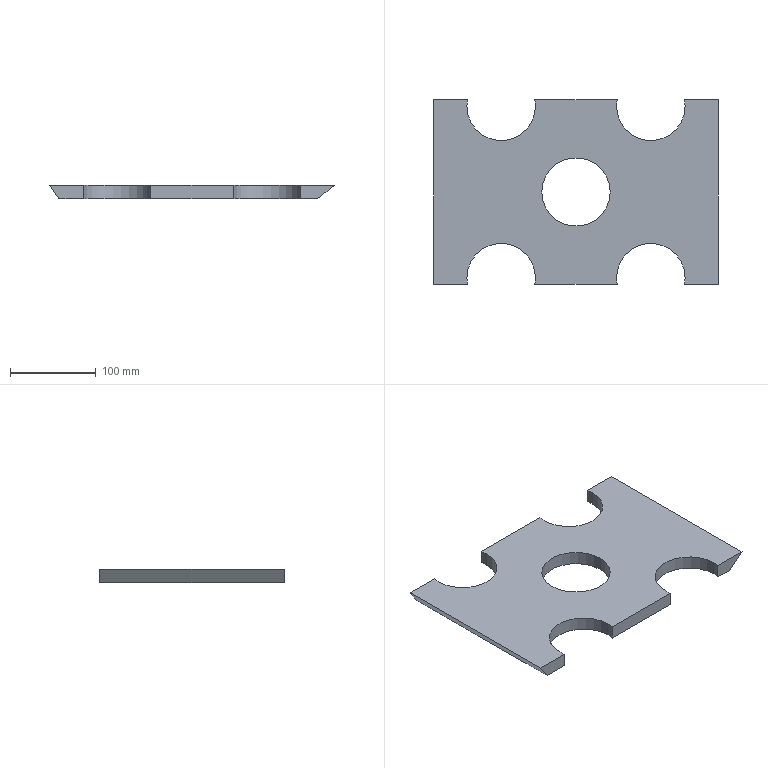Part | SolidWorks | features Extrusion 1, ICE 1 | 1 solid | 24 faces | box 333 x 216 x 16 mm | volume 816357 mm3 | cylinder 14 | plane 10 | commonest cylinder face diameters 80 x14
STEP:
#1=CARTESIAN_POINT('',(126.5,108.,16.));
#2=VERTEX_POINT('',#1);
#3=CARTESIAN_POINT('',(206.5,108.,16.));
#4=VERTEX_POINT('',#3);
#5=CARTESIAN_POINT('',(166.5,108.,16.));
#6=DIRECTION('',(0.,0.,1.));
#7=DIRECTION('',(1.,0.,0.));
#8=AXIS2_PLACEMENT_3D('',#5,#6,#7);
#9=CIRCLE('',#8,40.);
#10=EDGE_CURVE('',#2,#4,#9,.T.);
#11=ORIENTED_EDGE('',*,*,#10,.T.);
#12=CARTESIAN_POINT('',(206.5,108.,0.));
#13=VERTEX_POINT('',#12);
#14=CARTESIAN_POINT('',(206.5,108.,16.));
#15=DIRECTION('',(0.,0.,-1.));
#16=VECTOR('',#15,1000.);
#17=LINE('',#14,#16);
#18=EDGE_CURVE('',#4,#13,#17,.T.);
#19=ORIENTED_EDGE('',*,*,#18,.T.);
#20=CARTESIAN_POINT('',(126.5,108.,0.));
#21=VERTEX_POINT('',#20);
#22=CARTESIAN_POINT('',(166.5,108.,0.));
#23=DIRECTION('',(0.,0.,1.));
#24=DIRECTION('',(1.,0.,0.));
#25=AXIS2_PLACEMENT_3D('',#22,#23,#24);
#26=CIRCLE('',#25,40.);
#27=EDGE_CURVE('',#21,#13,#26,.T.);
#28=ORIENTED_EDGE('',*,*,#27,.F.);
#29=CARTESIAN_POINT('',(126.5,108.,16.));
#30=DIRECTION('',(0.,0.,-1.));
#31=VECTOR('',#30,1000.);
#32=LINE('',#29,#31);
#33=EDGE_CURVE('',#2,#21,#32,.T.);
#34=ORIENTED_EDGE('',*,*,#33,.F.);
#35=EDGE_LOOP('',(#11,#19,#28,#34));
#36=FACE_OUTER_BOUND('',#35,.T.);
#37=CARTESIAN_POINT('',(166.5,108.,16.));
#38=DIRECTION('',(0.,0.,-1.));
#39=DIRECTION('',(-1.,0.,0.));
#40=AXIS2_PLACEMENT_3D('',#37,#38,#39);
#41=CYLINDRICAL_SURFACE('',#40,40.);
#42=ADVANCED_FACE('',(#36),#41,.F.);
#43=CARTESIAN_POINT('',(119.,208.,16.));
#44=VERTEX_POINT('',#43);
#45=CARTESIAN_POINT('',(39.,208.,16.));
#46=VERTEX_POINT('',#45);
#47=CARTESIAN_POINT('',(79.,208.,16.));
#48=DIRECTION('',(0.,0.,-1.));
#49=DIRECTION('',(1.,0.,0.));
#50=AXIS2_PLACEMENT_3D('',#47,#48,#49);
#51=CIRCLE('',#50,40.);
#52=EDGE_CURVE('',#44,#46,#51,.T.);
#53=ORIENTED_EDGE('',*,*,#52,.F.);
#54=CARTESIAN_POINT('',(119.,208.,0.));
#55=VERTEX_POINT('',#54);
#56=CARTESIAN_POINT('',(119.,208.,16.));
#57=DIRECTION('',(0.,0.,-1.));
#58=VECTOR('',#57,1000.);
#59=LINE('',#56,#58);
#60=EDGE_CURVE('',#44,#55,#59,.T.);
#61=ORIENTED_EDGE('',*,*,#60,.T.);
#62=CARTESIAN_POINT('',(39.,208.,0.));
#63=VERTEX_POINT('',#62);
#64=CARTESIAN_POINT('',(79.,208.,0.));
#65=DIRECTION('',(0.,0.,-1.));
#66=DIRECTION('',(1.,0.,0.));
#67=AXIS2_PLACEMENT_3D('',#64,#65,#66);
#68=CIRCLE('',#67,40.);
#69=EDGE_CURVE('',#55,#63,#68,.T.);
#70=ORIENTED_EDGE('',*,*,#69,.T.);
#71=CARTESIAN_POINT('',(39.,208.,16.));
#72=DIRECTION('',(0.,0.,-1.));
#73=VECTOR('',#72,1000.);
#74=LINE('',#71,#73);
#75=EDGE_CURVE('',#46,#63,#74,.T.);
#76=ORIENTED_EDGE('',*,*,#75,.F.);
#77=EDGE_LOOP('',(#53,#61,#70,#76));
#78=FACE_OUTER_BOUND('',#77,.T.);
#79=CARTESIAN_POINT('',(79.,208.,16.));
#80=DIRECTION('',(0.,0.,-1.));
#81=DIRECTION('',(-1.,0.,0.));
#82=AXIS2_PLACEMENT_3D('',#79,#80,#81);
#83=CYLINDRICAL_SURFACE('',#82,40.);
#84=ADVANCED_FACE('',(#78),#83,.F.);
#85=CARTESIAN_POINT('',(39.808,216.,16.));
#86=VERTEX_POINT('',#85);
#87=CARTESIAN_POINT('',(79.,208.,16.));
#88=DIRECTION('',(0.,0.,-1.));
#89=DIRECTION('',(1.,0.,0.));
#90=AXIS2_PLACEMENT_3D('',#87,#88,#89);
#91=CIRCLE('',#90,40.);
#92=EDGE_CURVE('',#46,#86,#91,.T.);
#93=ORIENTED_EDGE('',*,*,#92,.F.);
#94=ORIENTED_EDGE('',*,*,#75,.T.);
#95=CARTESIAN_POINT('',(39.808,216.,0.));
#96=VERTEX_POINT('',#95);
#97=CARTESIAN_POINT('',(79.,208.,0.));
#98=DIRECTION('',(0.,0.,-1.));
#99=DIRECTION('',(1.,0.,0.));
#100=AXIS2_PLACEMENT_3D('',#97,#98,#99);
#101=CIRCLE('',#100,40.);
#102=EDGE_CURVE('',#63,#96,#101,.T.);
#103=ORIENTED_EDGE('',*,*,#102,.T.);
#104=CARTESIAN_POINT('',(39.808,216.,16.));
#105=DIRECTION('',(0.,0.,-1.));
#106=VECTOR('',#105,1000.);
#107=LINE('',#104,#106);
#108=EDGE_CURVE('',#86,#96,#107,.T.);
#109=ORIENTED_EDGE('',*,*,#108,.F.);
#110=EDGE_LOOP('',(#93,#94,#103,#109));
#111=FACE_OUTER_BOUND('',#110,.T.);
#112=CARTESIAN_POINT('',(79.,208.,16.));
#113=DIRECTION('',(0.,0.,-1.));
#114=DIRECTION('',(-1.,0.,0.));
#115=AXIS2_PLACEMENT_3D('',#112,#113,#114);
#116=CYLINDRICAL_SURFACE('',#115,40.);
#117=ADVANCED_FACE('',(#111),#116,.F.);
#118=CARTESIAN_POINT('',(294.,208.,16.));
#119=VERTEX_POINT('',#118);
#120=CARTESIAN_POINT('',(214.,208.,16.));
#121=VERTEX_POINT('',#120);
#122=CARTESIAN_POINT('',(254.,208.,16.));
#123=DIRECTION('',(0.,0.,-1.));
#124=DIRECTION('',(1.,0.,0.));
#125=AXIS2_PLACEMENT_3D('',#122,#123,#124);
#126=CIRCLE('',#125,40.);
#127=EDGE_CURVE('',#119,#121,#126,.T.);
#128=ORIENTED_EDGE('',*,*,#127,.F.);
#129=CARTESIAN_POINT('',(294.,208.,0.));
#130=VERTEX_POINT('',#129);
#131=CARTESIAN_POINT('',(294.,208.,16.));
#132=DIRECTION('',(0.,0.,-1.));
#133=VECTOR('',#132,1000.);
#134=LINE('',#131,#133);
#135=EDGE_CURVE('',#119,#130,#134,.T.);
#136=ORIENTED_EDGE('',*,*,#135,.T.);
#137=CARTESIAN_POINT('',(214.,208.,0.));
#138=VERTEX_POINT('',#137);
#139=CARTESIAN_POINT('',(254.,208.,0.));
#140=DIRECTION('',(0.,0.,-1.));
#141=DIRECTION('',(1.,0.,0.));
#142=AXIS2_PLACEMENT_3D('',#139,#140,#141);
#143=CIRCLE('',#142,40.);
#144=EDGE_CURVE('',#130,#138,#143,.T.);
#145=ORIENTED_EDGE('',*,*,#144,.T.);
#146=CARTESIAN_POINT('',(214.,208.,16.));
#147=DIRECTION('',(0.,0.,-1.));
#148=VECTOR('',#147,1000.);
#149=LINE('',#146,#148);
#150=EDGE_CURVE('',#121,#138,#149,.T.);
#151=ORIENTED_EDGE('',*,*,#150,.F.);
#152=EDGE_LOOP('',(#128,#136,#145,#151));
#153=FACE_OUTER_BOUND('',#152,.T.);
#154=CARTESIAN_POINT('',(254.,208.,16.));
#155=DIRECTION('',(0.,0.,-1.));
#156=DIRECTION('',(-1.,0.,0.));
#157=AXIS2_PLACEMENT_3D('',#154,#155,#156);
#158=CYLINDRICAL_SURFACE('',#157,40.);
#159=ADVANCED_FACE('',(#153),#158,.F.);
#160=CARTESIAN_POINT('',(214.808,216.,16.));
#161=VERTEX_POINT('',#160);
#162=CARTESIAN_POINT('',(254.,208.,16.));
#163=DIRECTION('',(0.,0.,-1.));
#164=DIRECTION('',(1.,0.,0.));
#165=AXIS2_PLACEMENT_3D('',#162,#163,#164);
#166=CIRCLE('',#165,40.);
#167=EDGE_CURVE('',#121,#161,#166,.T.);
#168=ORIENTED_EDGE('',*,*,#167,.F.);
#169=ORIENTED_EDGE('',*,*,#150,.T.);
#170=CARTESIAN_POINT('',(214.808,216.,0.));
#171=VERTEX_POINT('',#170);
#172=CARTESIAN_POINT('',(254.,208.,0.));
#173=DIRECTION('',(0.,0.,-1.));
#174=DIRECTION('',(1.,0.,0.));
#175=AXIS2_PLACEMENT_3D('',#172,#173,#174);
#176=CIRCLE('',#175,40.);
#177=EDGE_CURVE('',#138,#171,#176,.T.);
#178=ORIENTED_EDGE('',*,*,#177,.T.);
#179=CARTESIAN_POINT('',(214.808,216.,16.));
#180=DIRECTION('',(0.,0.,-1.));
#181=VECTOR('',#180,1000.);
#182=LINE('',#179,#181);
#183=EDGE_CURVE('',#161,#171,#182,.T.);
#184=ORIENTED_EDGE('',*,*,#183,.F.);
#185=EDGE_LOOP('',(#168,#169,#178,#184));
#186=FACE_OUTER_BOUND('',#185,.T.);
#187=CARTESIAN_POINT('',(254.,208.,16.));
#188=DIRECTION('',(0.,0.,-1.));
#189=DIRECTION('',(-1.,0.,0.));
#190=AXIS2_PLACEMENT_3D('',#187,#188,#189);
#191=CYLINDRICAL_SURFACE('',#190,40.);
#192=ADVANCED_FACE('',(#186),#191,.F.);
#193=CARTESIAN_POINT('',(294.,8.,16.));
#194=VERTEX_POINT('',#193);
#195=CARTESIAN_POINT('',(293.192,0.,16.));
#196=VERTEX_POINT('',#195);
#197=CARTESIAN_POINT('',(254.,8.,16.));
#198=DIRECTION('',(0.,0.,-1.));
#199=DIRECTION('',(1.,0.,0.));
#200=AXIS2_PLACEMENT_3D('',#197,#198,#199);
#201=CIRCLE('',#200,40.);
#202=EDGE_CURVE('',#194,#196,#201,.T.);
#203=ORIENTED_EDGE('',*,*,#202,.F.);
#204=CARTESIAN_POINT('',(294.,8.,0.));
#205=VERTEX_POINT('',#204);
#206=CARTESIAN_POINT('',(294.,8.,16.));
#207=DIRECTION('',(0.,0.,-1.));
#208=VECTOR('',#207,1000.);
#209=LINE('',#206,#208);
#210=EDGE_CURVE('',#194,#205,#209,.T.);
#211=ORIENTED_EDGE('',*,*,#210,.T.);
#212=CARTESIAN_POINT('',(293.192,0.,0.));
#213=VERTEX_POINT('',#212);
#214=CARTESIAN_POINT('',(254.,8.,0.));
#215=DIRECTION('',(0.,0.,-1.));
#216=DIRECTION('',(1.,0.,0.));
#217=AXIS2_PLACEMENT_3D('',#214,#215,#216);
#218=CIRCLE('',#217,40.);
#219=EDGE_CURVE('',#205,#213,#218,.T.);
#220=ORIENTED_EDGE('',*,*,#219,.T.);
#221=CARTESIAN_POINT('',(293.192,0.,16.));
#222=DIRECTION('',(0.,0.,-1.));
#223=VECTOR('',#222,1000.);
#224=LINE('',#221,#223);
#225=EDGE_CURVE('',#196,#213,#224,.T.);
#226=ORIENTED_EDGE('',*,*,#225,.F.);
#227=EDGE_LOOP('',(#203,#211,#220,#226));
#228=FACE_OUTER_BOUND('',#227,.T.);
#229=CARTESIAN_POINT('',(254.,8.,16.));
#230=DIRECTION('',(0.,0.,-1.));
#231=DIRECTION('',(-1.,0.,0.));
#232=AXIS2_PLACEMENT_3D('',#229,#230,#231);
#233=CYLINDRICAL_SURFACE('',#232,40.);
#234=ADVANCED_FACE('',(#228),#233,.F.);
#235=ORIENTED_EDGE('',*,*,#210,.F.);
#236=CARTESIAN_POINT('',(214.,8.,16.));
#237=VERTEX_POINT('',#236);
#238=CARTESIAN_POINT('',(254.,8.,16.));
#239=DIRECTION('',(0.,0.,-1.));
#240=DIRECTION('',(1.,0.,0.));
#241=AXIS2_PLACEMENT_3D('',#238,#239,#240);
#242=CIRCLE('',#241,40.);
#243=EDGE_CURVE('',#237,#194,#242,.T.);
#244=ORIENTED_EDGE('',*,*,#243,.F.);
#245=CARTESIAN_POINT('',(214.,8.,0.));
#246=VERTEX_POINT('',#245);
#247=CARTESIAN_POINT('',(214.,8.,16.));
#248=DIRECTION('',(0.,0.,-1.));
#249=VECTOR('',#248,1000.);
#250=LINE('',#247,#249);
#251=EDGE_CURVE('',#237,#246,#250,.T.);
#252=ORIENTED_EDGE('',*,*,#251,.T.);
#253=CARTESIAN_POINT('',(254.,8.,0.));
#254=DIRECTION('',(0.,0.,-1.));
#255=DIRECTION('',(1.,0.,0.));
#256=AXIS2_PLACEMENT_3D('',#253,#254,#255);
#257=CIRCLE('',#256,40.);
#258=EDGE_CURVE('',#246,#205,#257,.T.);
#259=ORIENTED_EDGE('',*,*,#258,.T.);
#260=EDGE_LOOP('',(#235,#244,#252,#259));
#261=FACE_OUTER_BOUND('',#260,.T.);
#262=CARTESIAN_POINT('',(254.,8.,16.));
#263=DIRECTION('',(0.,0.,-1.));
#264=DIRECTION('',(-1.,0.,0.));
#265=AXIS2_PLACEMENT_3D('',#262,#263,#264);
#266=CYLINDRICAL_SURFACE('',#265,40.);
#267=ADVANCED_FACE('',(#261),#266,.F.);
#268=CARTESIAN_POINT('',(119.,8.,16.));
#269=VERTEX_POINT('',#268);
#270=CARTESIAN_POINT('',(118.192,0.,16.));
#271=VERTEX_POINT('',#270);
#272=CARTESIAN_POINT('',(79.,8.,16.));
#273=DIRECTION('',(0.,0.,-1.));
#274=DIRECTION('',(1.,0.,0.));
#275=AXIS2_PLACEMENT_3D('',#272,#273,#274);
#276=CIRCLE('',#275,40.);
#277=EDGE_CURVE('',#269,#271,#276,.T.);
#278=ORIENTED_EDGE('',*,*,#277,.F.);
#279=CARTESIAN_POINT('',(119.,8.,0.));
#280=VERTEX_POINT('',#279);
#281=CARTESIAN_POINT('',(119.,8.,16.));
#282=DIRECTION('',(0.,0.,-1.));
#283=VECTOR('',#282,1000.);
#284=LINE('',#281,#283);
#285=EDGE_CURVE('',#269,#280,#284,.T.);
#286=ORIENTED_EDGE('',*,*,#285,.T.);
#287=CARTESIAN_POINT('',(118.192,0.,0.));
#288=VERTEX_POINT('',#287);
#289=CARTESIAN_POINT('',(79.,8.,0.));
#290=DIRECTION('',(0.,0.,-1.));
#291=DIRECTION('',(1.,0.,0.));
#292=AXIS2_PLACEMENT_3D('',#289,#290,#291);
#293=CIRCLE('',#292,40.);
#294=EDGE_CURVE('',#280,#288,#293,.T.);
#295=ORIENTED_EDGE('',*,*,#294,.T.);
#296=CARTESIAN_POINT('',(118.192,0.,16.));
#297=DIRECTION('',(0.,0.,-1.));
#298=VECTOR('',#297,1000.);
#299=LINE('',#296,#298);
#300=EDGE_CURVE('',#271,#288,#299,.T.);
#301=ORIENTED_EDGE('',*,*,#300,.F.);
#302=EDGE_LOOP('',(#278,#286,#295,#301));
#303=FACE_OUTER_BOUND('',#302,.T.);
#304=CARTESIAN_POINT('',(79.,8.,16.));
#305=DIRECTION('',(0.,0.,-1.));
#306=DIRECTION('',(-1.,0.,0.));
#307=AXIS2_PLACEMENT_3D('',#304,#305,#306);
#308=CYLINDRICAL_SURFACE('',#307,40.);
#309=ADVANCED_FACE('',(#303),#308,.F.);
#310=ORIENTED_EDGE('',*,*,#285,.F.);
#311=CARTESIAN_POINT('',(39.,8.,16.));
#312=VERTEX_POINT('',#311);
#313=CARTESIAN_POINT('',(79.,8.,16.));
#314=DIRECTION('',(0.,0.,-1.));
#315=DIRECTION('',(1.,0.,0.));
#316=AXIS2_PLACEMENT_3D('',#313,#314,#315);
#317=CIRCLE('',#316,40.);
#318=EDGE_CURVE('',#312,#269,#317,.T.);
#319=ORIENTED_EDGE('',*,*,#318,.F.);
#320=CARTESIAN_POINT('',(39.,8.,0.));
#321=VERTEX_POINT('',#320);
#322=CARTESIAN_POINT('',(39.,8.,16.));
#323=DIRECTION('',(0.,0.,-1.));
#324=VECTOR('',#323,1000.);
#325=LINE('',#322,#324);
#326=EDGE_CURVE('',#312,#321,#325,.T.);
#327=ORIENTED_EDGE('',*,*,#326,.T.);
#328=CARTESIAN_POINT('',(79.,8.,0.));
#329=DIRECTION('',(0.,0.,-1.));
#330=DIRECTION('',(1.,0.,0.));
#331=AXIS2_PLACEMENT_3D('',#328,#329,#330);
#332=CIRCLE('',#331,40.);
#333=EDGE_CURVE('',#321,#280,#332,.T.);
#334=ORIENTED_EDGE('',*,*,#333,.T.);
#335=EDGE_LOOP('',(#310,#319,#327,#334));
#336=FACE_OUTER_BOUND('',#335,.T.);
#337=CARTESIAN_POINT('',(79.,8.,16.));
#338=DIRECTION('',(0.,0.,-1.));
#339=DIRECTION('',(-1.,0.,0.));
#340=AXIS2_PLACEMENT_3D('',#337,#338,#339);
#341=CYLINDRICAL_SURFACE('',#340,40.);
#342=ADVANCED_FACE('',(#336),#341,.F.);
#343=CARTESIAN_POINT('',(0.,216.,16.));
#344=VERTEX_POINT('',#343);
#345=CARTESIAN_POINT('',(0.,0.,16.));
#346=VERTEX_POINT('',#345);
#347=CARTESIAN_POINT('',(0.,0.,16.));
#348=DIRECTION('',(0.,-1.,0.));
#349=VECTOR('',#348,1000.);
#350=LINE('',#347,#349);
#351=EDGE_CURVE('',#344,#346,#350,.T.);
#352=ORIENTED_EDGE('',*,*,#351,.T.);
#353=CARTESIAN_POINT('',(39.808,0.,16.));
#354=VERTEX_POINT('',#353);
#355=CARTESIAN_POINT('',(0.,0.,16.));
#356=DIRECTION('',(1.,0.,0.));
#357=VECTOR('',#356,1000.);
#358=LINE('',#355,#357);
#359=EDGE_CURVE('',#346,#354,#358,.T.);
#360=ORIENTED_EDGE('',*,*,#359,.T.);
#361=CARTESIAN_POINT('',(79.,8.,16.));
#362=DIRECTION('',(0.,0.,-1.));
#363=DIRECTION('',(1.,0.,0.));
#364=AXIS2_PLACEMENT_3D('',#361,#362,#363);
#365=CIRCLE('',#364,40.);
#366=EDGE_CURVE('',#354,#312,#365,.T.);
#367=ORIENTED_EDGE('',*,*,#366,.T.);
#368=ORIENTED_EDGE('',*,*,#318,.T.);
#369=ORIENTED_EDGE('',*,*,#277,.T.);
#370=CARTESIAN_POINT('',(214.808,0.,16.));
#371=VERTEX_POINT('',#370);
#372=CARTESIAN_POINT('',(118.192,0.,16.));
#373=DIRECTION('',(1.,0.,0.));
#374=VECTOR('',#373,1000.);
#375=LINE('',#372,#374);
#376=EDGE_CURVE('',#271,#371,#375,.T.);
#377=ORIENTED_EDGE('',*,*,#376,.T.);
#378=CARTESIAN_POINT('',(254.,8.,16.));
#379=DIRECTION('',(0.,0.,-1.));
#380=DIRECTION('',(1.,0.,0.));
#381=AXIS2_PLACEMENT_3D('',#378,#379,#380);
#382=CIRCLE('',#381,40.);
#383=EDGE_CURVE('',#371,#237,#382,.T.);
#384=ORIENTED_EDGE('',*,*,#383,.T.);
#385=ORIENTED_EDGE('',*,*,#243,.T.);
#386=ORIENTED_EDGE('',*,*,#202,.T.);
#387=CARTESIAN_POINT('',(333.,0.,16.));
#388=VERTEX_POINT('',#387);
#389=CARTESIAN_POINT('',(293.192,0.,16.));
#390=DIRECTION('',(1.,0.,0.));
#391=VECTOR('',#390,1000.);
#392=LINE('',#389,#391);
#393=EDGE_CURVE('',#196,#388,#392,.T.);
#394=ORIENTED_EDGE('',*,*,#393,.T.);
#395=CARTESIAN_POINT('',(333.,216.,16.));
#396=VERTEX_POINT('',#395);
#397=CARTESIAN_POINT('',(333.,0.,16.));
#398=DIRECTION('',(0.,1.,0.));
#399=VECTOR('',#398,1000.);
#400=LINE('',#397,#399);
#401=EDGE_CURVE('',#388,#396,#400,.T.);
#402=ORIENTED_EDGE('',*,*,#401,.T.);
#403=CARTESIAN_POINT('',(293.192,216.,16.));
#404=VERTEX_POINT('',#403);
#405=CARTESIAN_POINT('',(293.192,216.,16.));
#406=DIRECTION('',(-1.,0.,0.));
#407=VECTOR('',#406,1000.);
#408=LINE('',#405,#407);
#409=EDGE_CURVE('',#396,#404,#408,.T.);
#410=ORIENTED_EDGE('',*,*,#409,.T.);
#411=CARTESIAN_POINT('',(254.,208.,16.));
#412=DIRECTION('',(0.,0.,-1.));
#413=DIRECTION('',(1.,0.,0.));
#414=AXIS2_PLACEMENT_3D('',#411,#412,#413);
#415=CIRCLE('',#414,40.);
#416=EDGE_CURVE('',#404,#119,#415,.T.);
#417=ORIENTED_EDGE('',*,*,#416,.T.);
#418=ORIENTED_EDGE('',*,*,#127,.T.);
#419=ORIENTED_EDGE('',*,*,#167,.T.);
#420=CARTESIAN_POINT('',(118.192,216.,16.));
#421=VERTEX_POINT('',#420);
#422=CARTESIAN_POINT('',(118.192,216.,16.));
#423=DIRECTION('',(-1.,0.,0.));
#424=VECTOR('',#423,1000.);
#425=LINE('',#422,#424);
#426=EDGE_CURVE('',#161,#421,#425,.T.);
#427=ORIENTED_EDGE('',*,*,#426,.T.);
#428=CARTESIAN_POINT('',(79.,208.,16.));
#429=DIRECTION('',(0.,0.,-1.));
#430=DIRECTION('',(1.,0.,0.));
#431=AXIS2_PLACEMENT_3D('',#428,#429,#430);
#432=CIRCLE('',#431,40.);
#433=EDGE_CURVE('',#421,#44,#432,.T.);
#434=ORIENTED_EDGE('',*,*,#433,.T.);
#435=ORIENTED_EDGE('',*,*,#52,.T.);
#436=ORIENTED_EDGE('',*,*,#92,.T.);
#437=CARTESIAN_POINT('',(0.,216.,16.));
#438=DIRECTION('',(-1.,0.,0.));
#439=VECTOR('',#438,1000.);
#440=LINE('',#437,#439);
#441=EDGE_CURVE('',#86,#344,#440,.T.);
#442=ORIENTED_EDGE('',*,*,#441,.T.);
#443=EDGE_LOOP('',(#352,#360,#367,#368,#369,#377,#384,#385,#386,#394,#402,#410,#417,#418,#419,#427,#434,#435,#436,#442));
#444=FACE_OUTER_BOUND('',#443,.T.);
#445=ORIENTED_EDGE('',*,*,#10,.F.);
#446=CARTESIAN_POINT('',(166.5,108.,16.));
#447=DIRECTION('',(0.,0.,1.));
#448=DIRECTION('',(1.,0.,0.));
#449=AXIS2_PLACEMENT_3D('',#446,#447,#448);
#450=CIRCLE('',#449,40.);
#451=EDGE_CURVE('',#4,#2,#450,.T.);
#452=ORIENTED_EDGE('',*,*,#451,.F.);
#453=EDGE_LOOP('',(#445,#452));
#454=FACE_BOUND('',#453,.T.);
#455=CARTESIAN_POINT('',(79.,208.,16.));
#456=DIRECTION('',(0.,0.,1.));
#457=DIRECTION('',(1.,0.,0.));
#458=AXIS2_PLACEMENT_3D('',#455,#456,#457);
#459=PLANE('',#458);
#460=ADVANCED_FACE('',(#444,#454),#459,.T.);
#461=CARTESIAN_POINT('',(313.3,216.,0.));
#462=VERTEX_POINT('',#461);
#463=CARTESIAN_POINT('',(293.192,216.,0.));
#464=VERTEX_POINT('',#463);
#465=CARTESIAN_POINT('',(293.192,216.,0.));
#466=DIRECTION('',(-1.,0.,0.));
#467=VECTOR('',#466,1000.);
#468=LINE('',#465,#467);
#469=EDGE_CURVE('',#462,#464,#468,.T.);
#470=ORIENTED_EDGE('',*,*,#469,.F.);
#471=CARTESIAN_POINT('',(313.3,0.,0.));
#472=VERTEX_POINT('',#471);
#473=CARTESIAN_POINT('',(313.3,216.,0.));
#474=DIRECTION('',(0.,-1.,0.));
#475=VECTOR('',#474,1000.);
#476=LINE('',#473,#475);
#477=EDGE_CURVE('',#462,#472,#476,.T.);
#478=ORIENTED_EDGE('',*,*,#477,.T.);
#479=CARTESIAN_POINT('',(293.192,0.,0.));
#480=DIRECTION('',(1.,0.,0.));
#481=VECTOR('',#480,1000.);
#482=LINE('',#479,#481);
#483=EDGE_CURVE('',#213,#472,#482,.T.);
#484=ORIENTED_EDGE('',*,*,#483,.F.);
#485=ORIENTED_EDGE('',*,*,#219,.F.);
#486=ORIENTED_EDGE('',*,*,#258,.F.);
#487=CARTESIAN_POINT('',(214.808,0.,0.));
#488=VERTEX_POINT('',#487);
#489=CARTESIAN_POINT('',(254.,8.,0.));
#490=DIRECTION('',(0.,0.,-1.));
#491=DIRECTION('',(1.,0.,0.));
#492=AXIS2_PLACEMENT_3D('',#489,#490,#491);
#493=CIRCLE('',#492,40.);
#494=EDGE_CURVE('',#488,#246,#493,.T.);
#495=ORIENTED_EDGE('',*,*,#494,.F.);
#496=CARTESIAN_POINT('',(118.192,0.,0.));
#497=DIRECTION('',(1.,0.,0.));
#498=VECTOR('',#497,1000.);
#499=LINE('',#496,#498);
#500=EDGE_CURVE('',#288,#488,#499,.T.);
#501=ORIENTED_EDGE('',*,*,#500,.F.);
#502=ORIENTED_EDGE('',*,*,#294,.F.);
#503=ORIENTED_EDGE('',*,*,#333,.F.);
#504=CARTESIAN_POINT('',(39.808,0.,0.));
#505=VERTEX_POINT('',#504);
#506=CARTESIAN_POINT('',(79.,8.,0.));
#507=DIRECTION('',(0.,0.,-1.));
#508=DIRECTION('',(1.,0.,0.));
#509=AXIS2_PLACEMENT_3D('',#506,#507,#508);
#510=CIRCLE('',#509,40.);
#511=EDGE_CURVE('',#505,#321,#510,.T.);
#512=ORIENTED_EDGE('',*,*,#511,.F.);
#513=CARTESIAN_POINT('',(10.7,0.,0.));
#514=VERTEX_POINT('',#513);
#515=CARTESIAN_POINT('',(0.,0.,0.));
#516=DIRECTION('',(1.,0.,0.));
#517=VECTOR('',#516,1000.);
#518=LINE('',#515,#517);
#519=EDGE_CURVE('',#514,#505,#518,.T.);
#520=ORIENTED_EDGE('',*,*,#519,.F.);
#521=CARTESIAN_POINT('',(10.7,216.,0.));
#522=VERTEX_POINT('',#521);
#523=CARTESIAN_POINT('',(10.7,216.,0.));
#524=DIRECTION('',(0.,-1.,0.));
#525=VECTOR('',#524,1000.);
#526=LINE('',#523,#525);
#527=EDGE_CURVE('',#522,#514,#526,.T.);
#528=ORIENTED_EDGE('',*,*,#527,.F.);
#529=CARTESIAN_POINT('',(0.,216.,0.));
#530=DIRECTION('',(-1.,0.,0.));
#531=VECTOR('',#530,1000.);
#532=LINE('',#529,#531);
#533=EDGE_CURVE('',#96,#522,#532,.T.);
#534=ORIENTED_EDGE('',*,*,#533,.F.);
#535=ORIENTED_EDGE('',*,*,#102,.F.);
#536=ORIENTED_EDGE('',*,*,#69,.F.);
#537=CARTESIAN_POINT('',(118.192,216.,0.));
#538=VERTEX_POINT('',#537);
#539=CARTESIAN_POINT('',(79.,208.,0.));
#540=DIRECTION('',(0.,0.,-1.));
#541=DIRECTION('',(1.,0.,0.));
#542=AXIS2_PLACEMENT_3D('',#539,#540,#541);
#543=CIRCLE('',#542,40.);
#544=EDGE_CURVE('',#538,#55,#543,.T.);
#545=ORIENTED_EDGE('',*,*,#544,.F.);
#546=CARTESIAN_POINT('',(118.192,216.,0.));
#547=DIRECTION('',(-1.,0.,0.));
#548=VECTOR('',#547,1000.);
#549=LINE('',#546,#548);
#550=EDGE_CURVE('',#171,#538,#549,.T.);
#551=ORIENTED_EDGE('',*,*,#550,.F.);
#552=ORIENTED_EDGE('',*,*,#177,.F.);
#553=ORIENTED_EDGE('',*,*,#144,.F.);
#554=CARTESIAN_POINT('',(254.,208.,0.));
#555=DIRECTION('',(0.,0.,-1.));
#556=DIRECTION('',(1.,0.,0.));
#557=AXIS2_PLACEMENT_3D('',#554,#555,#556);
#558=CIRCLE('',#557,40.);
#559=EDGE_CURVE('',#464,#130,#558,.T.);
#560=ORIENTED_EDGE('',*,*,#559,.F.);
#561=EDGE_LOOP('',(#470,#478,#484,#485,#486,#495,#501,#502,#503,#512,#520,#528,#534,#535,#536,#545,#551,#552,#553,#560));
#562=FACE_OUTER_BOUND('',#561,.T.);
#563=ORIENTED_EDGE('',*,*,#27,.T.);
#564=CARTESIAN_POINT('',(166.5,108.,0.));
#565=DIRECTION('',(0.,0.,1.));
#566=DIRECTION('',(1.,0.,0.));
#567=AXIS2_PLACEMENT_3D('',#564,#565,#566);
#568=CIRCLE('',#567,40.);
#569=EDGE_CURVE('',#13,#21,#568,.T.);
#570=ORIENTED_EDGE('',*,*,#569,.T.);
#571=EDGE_LOOP('',(#563,#570));
#572=FACE_BOUND('',#571,.T.);
#573=CARTESIAN_POINT('',(79.,208.,0.));
#574=DIRECTION('',(0.,0.,1.));
#575=DIRECTION('',(1.,0.,0.));
#576=AXIS2_PLACEMENT_3D('',#573,#574,#575);
#577=PLANE('',#576);
#578=ADVANCED_FACE('',(#562,#572),#577,.F.);
#579=ORIENTED_EDGE('',*,*,#359,.F.);
#580=CARTESIAN_POINT('',(0.,0.,16.));
#581=DIRECTION('',(-0.5559,0.,0.8313));
#582=VECTOR('',#581,1000.);
#583=LINE('',#580,#582);
#584=EDGE_CURVE('',#514,#346,#583,.T.);
#585=ORIENTED_EDGE('',*,*,#584,.F.);
#586=ORIENTED_EDGE('',*,*,#519,.T.);
#587=CARTESIAN_POINT('',(39.808,0.,16.));
#588=DIRECTION('',(0.,0.,-1.));
#589=VECTOR('',#588,1000.);
#590=LINE('',#587,#589);
#591=EDGE_CURVE('',#354,#505,#590,.T.);
#592=ORIENTED_EDGE('',*,*,#591,.F.);
#593=EDGE_LOOP('',(#579,#585,#586,#592));
#594=FACE_OUTER_BOUND('',#593,.T.);
#595=CARTESIAN_POINT('',(0.,0.,16.));
#596=DIRECTION('',(0.,1.,0.));
#597=DIRECTION('',(0.,0.,1.));
#598=AXIS2_PLACEMENT_3D('',#595,#596,#597);
#599=PLANE('',#598);
#600=ADVANCED_FACE('',(#594),#599,.F.);
#601=ORIENTED_EDGE('',*,*,#326,.F.);
#602=ORIENTED_EDGE('',*,*,#366,.F.);
#603=ORIENTED_EDGE('',*,*,#591,.T.);
#604=ORIENTED_EDGE('',*,*,#511,.T.);
#605=EDGE_LOOP('',(#601,#602,#603,#604));
#606=FACE_OUTER_BOUND('',#605,.T.);
#607=CARTESIAN_POINT('',(79.,8.,16.));
#608=DIRECTION('',(0.,0.,-1.));
#609=DIRECTION('',(-1.,0.,0.));
#610=AXIS2_PLACEMENT_3D('',#607,#608,#609);
#611=CYLINDRICAL_SURFACE('',#610,40.);
#612=ADVANCED_FACE('',(#606),#611,.F.);
#613=ORIENTED_EDGE('',*,*,#500,.T.);
#614=CARTESIAN_POINT('',(214.808,0.,16.));
#615=DIRECTION('',(0.,0.,-1.));
#616=VECTOR('',#615,1000.);
#617=LINE('',#614,#616);
#618=EDGE_CURVE('',#371,#488,#617,.T.);
#619=ORIENTED_EDGE('',*,*,#618,.F.);
#620=ORIENTED_EDGE('',*,*,#376,.F.);
#621=ORIENTED_EDGE('',*,*,#300,.T.);
#622=EDGE_LOOP('',(#613,#619,#620,#621));
#623=FACE_OUTER_BOUND('',#622,.T.);
#624=CARTESIAN_POINT('',(118.192,0.,16.));
#625=DIRECTION('',(0.,1.,0.));
#626=DIRECTION('',(0.,0.,1.));
#627=AXIS2_PLACEMENT_3D('',#624,#625,#626);
#628=PLANE('',#627);
#629=ADVANCED_FACE('',(#623),#628,.F.);
#630=ORIENTED_EDGE('',*,*,#251,.F.);
#631=ORIENTED_EDGE('',*,*,#383,.F.);
#632=ORIENTED_EDGE('',*,*,#618,.T.);
#633=ORIENTED_EDGE('',*,*,#494,.T.);
#634=EDGE_LOOP('',(#630,#631,#632,#633));
#635=FACE_OUTER_BOUND('',#634,.T.);
#636=CARTESIAN_POINT('',(254.,8.,16.));
#637=DIRECTION('',(0.,0.,-1.));
#638=DIRECTION('',(-1.,0.,0.));
#639=AXIS2_PLACEMENT_3D('',#636,#637,#638);
#640=CYLINDRICAL_SURFACE('',#639,40.);
#641=ADVANCED_FACE('',(#635),#640,.F.);
#642=ORIENTED_EDGE('',*,*,#483,.T.);
#643=CARTESIAN_POINT('',(333.,0.,16.));
#644=DIRECTION('',(-0.7762,0.,-0.6304));
#645=VECTOR('',#644,1000.);
#646=LINE('',#643,#645);
#647=EDGE_CURVE('',#388,#472,#646,.T.);
#648=ORIENTED_EDGE('',*,*,#647,.F.);
#649=ORIENTED_EDGE('',*,*,#393,.F.);
#650=ORIENTED_EDGE('',*,*,#225,.T.);
#651=EDGE_LOOP('',(#642,#648,#649,#650));
#652=FACE_OUTER_BOUND('',#651,.T.);
#653=CARTESIAN_POINT('',(293.192,0.,16.));
#654=DIRECTION('',(0.,1.,0.));
#655=DIRECTION('',(0.,0.,1.));
#656=AXIS2_PLACEMENT_3D('',#653,#654,#655);
#657=PLANE('',#656);
#658=ADVANCED_FACE('',(#652),#657,.F.);
#659=ORIENTED_EDGE('',*,*,#409,.F.);
#660=CARTESIAN_POINT('',(333.,216.,16.));
#661=DIRECTION('',(-0.7762,0.,-0.6304));
#662=VECTOR('',#661,1000.);
#663=LINE('',#660,#662);
#664=EDGE_CURVE('',#396,#462,#663,.T.);
#665=ORIENTED_EDGE('',*,*,#664,.T.);
#666=ORIENTED_EDGE('',*,*,#469,.T.);
#667=CARTESIAN_POINT('',(293.192,216.,16.));
#668=DIRECTION('',(0.,0.,-1.));
#669=VECTOR('',#668,1000.);
#670=LINE('',#667,#669);
#671=EDGE_CURVE('',#404,#464,#670,.T.);
#672=ORIENTED_EDGE('',*,*,#671,.F.);
#673=EDGE_LOOP('',(#659,#665,#666,#672));
#674=FACE_OUTER_BOUND('',#673,.T.);
#675=CARTESIAN_POINT('',(293.192,216.,16.));
#676=DIRECTION('',(0.,-1.,0.));
#677=DIRECTION('',(0.,0.,-1.));
#678=AXIS2_PLACEMENT_3D('',#675,#676,#677);
#679=PLANE('',#678);
#680=ADVANCED_FACE('',(#674),#679,.F.);
#681=ORIENTED_EDGE('',*,*,#135,.F.);
#682=ORIENTED_EDGE('',*,*,#416,.F.);
#683=ORIENTED_EDGE('',*,*,#671,.T.);
#684=ORIENTED_EDGE('',*,*,#559,.T.);
#685=EDGE_LOOP('',(#681,#682,#683,#684));
#686=FACE_OUTER_BOUND('',#685,.T.);
#687=CARTESIAN_POINT('',(254.,208.,16.));
#688=DIRECTION('',(0.,0.,-1.));
#689=DIRECTION('',(-1.,0.,0.));
#690=AXIS2_PLACEMENT_3D('',#687,#688,#689);
#691=CYLINDRICAL_SURFACE('',#690,40.);
#692=ADVANCED_FACE('',(#686),#691,.F.);
#693=ORIENTED_EDGE('',*,*,#550,.T.);
#694=CARTESIAN_POINT('',(118.192,216.,16.));
#695=DIRECTION('',(0.,0.,-1.));
#696=VECTOR('',#695,1000.);
#697=LINE('',#694,#696);
#698=EDGE_CURVE('',#421,#538,#697,.T.);
#699=ORIENTED_EDGE('',*,*,#698,.F.);
#700=ORIENTED_EDGE('',*,*,#426,.F.);
#701=ORIENTED_EDGE('',*,*,#183,.T.);
#702=EDGE_LOOP('',(#693,#699,#700,#701));
#703=FACE_OUTER_BOUND('',#702,.T.);
#704=CARTESIAN_POINT('',(118.192,216.,16.));
#705=DIRECTION('',(0.,-1.,0.));
#706=DIRECTION('',(0.,0.,-1.));
#707=AXIS2_PLACEMENT_3D('',#704,#705,#706);
#708=PLANE('',#707);
#709=ADVANCED_FACE('',(#703),#708,.F.);
#710=ORIENTED_EDGE('',*,*,#60,.F.);
#711=ORIENTED_EDGE('',*,*,#433,.F.);
#712=ORIENTED_EDGE('',*,*,#698,.T.);
#713=ORIENTED_EDGE('',*,*,#544,.T.);
#714=EDGE_LOOP('',(#710,#711,#712,#713));
#715=FACE_OUTER_BOUND('',#714,.T.);
#716=CARTESIAN_POINT('',(79.,208.,16.));
#717=DIRECTION('',(0.,0.,-1.));
#718=DIRECTION('',(-1.,0.,0.));
#719=AXIS2_PLACEMENT_3D('',#716,#717,#718);
#720=CYLINDRICAL_SURFACE('',#719,40.);
#721=ADVANCED_FACE('',(#715),#720,.F.);
#722=ORIENTED_EDGE('',*,*,#533,.T.);
#723=CARTESIAN_POINT('',(0.,216.,16.));
#724=DIRECTION('',(-0.5559,0.,0.8313));
#725=VECTOR('',#724,1000.);
#726=LINE('',#723,#725);
#727=EDGE_CURVE('',#522,#344,#726,.T.);
#728=ORIENTED_EDGE('',*,*,#727,.T.);
#729=ORIENTED_EDGE('',*,*,#441,.F.);
#730=ORIENTED_EDGE('',*,*,#108,.T.);
#731=EDGE_LOOP('',(#722,#728,#729,#730));
#732=FACE_OUTER_BOUND('',#731,.T.);
#733=CARTESIAN_POINT('',(0.,216.,16.));
#734=DIRECTION('',(0.,-1.,0.));
#735=DIRECTION('',(0.,0.,-1.));
#736=AXIS2_PLACEMENT_3D('',#733,#734,#735);
#737=PLANE('',#736);
#738=ADVANCED_FACE('',(#732),#737,.F.);
#739=ORIENTED_EDGE('',*,*,#18,.F.);
#740=ORIENTED_EDGE('',*,*,#451,.T.);
#741=ORIENTED_EDGE('',*,*,#33,.T.);
#742=ORIENTED_EDGE('',*,*,#569,.F.);
#743=EDGE_LOOP('',(#739,#740,#741,#742));
#744=FACE_OUTER_BOUND('',#743,.T.);
#745=CARTESIAN_POINT('',(166.5,108.,16.));
#746=DIRECTION('',(0.,0.,-1.));
#747=DIRECTION('',(-1.,0.,0.));
#748=AXIS2_PLACEMENT_3D('',#745,#746,#747);
#749=CYLINDRICAL_SURFACE('',#748,40.);
#750=ADVANCED_FACE('',(#744),#749,.F.);
#751=ORIENTED_EDGE('',*,*,#584,.T.);
#752=ORIENTED_EDGE('',*,*,#351,.F.);
#753=ORIENTED_EDGE('',*,*,#727,.F.);
#754=ORIENTED_EDGE('',*,*,#527,.T.);
#755=EDGE_LOOP('',(#751,#752,#753,#754));
#756=FACE_OUTER_BOUND('',#755,.T.);
#757=CARTESIAN_POINT('',(0.,216.,16.));
#758=DIRECTION('',(0.8313,0.,0.5559));
#759=DIRECTION('',(0.5559,0.,-0.8313));
#760=AXIS2_PLACEMENT_3D('',#757,#758,#759);
#761=PLANE('',#760);
#762=ADVANCED_FACE('',(#756),#761,.F.);
#763=ORIENTED_EDGE('',*,*,#647,.T.);
#764=ORIENTED_EDGE('',*,*,#477,.F.);
#765=ORIENTED_EDGE('',*,*,#664,.F.);
#766=ORIENTED_EDGE('',*,*,#401,.F.);
#767=EDGE_LOOP('',(#763,#764,#765,#766));
#768=FACE_OUTER_BOUND('',#767,.T.);
#769=CARTESIAN_POINT('',(333.,216.,16.));
#770=DIRECTION('',(-0.6304,0.,0.7762));
#771=DIRECTION('',(0.7762,0.,0.6304));
#772=AXIS2_PLACEMENT_3D('',#769,#770,#771);
#773=PLANE('',#772);
#774=ADVANCED_FACE('',(#768),#773,.F.);
#775=CLOSED_SHELL('',(#42,#84,#117,#159,#192,#234,#267,#309,#342,#460,#578,#600,#612,#629,#641,#658,#680,#692,#709,#721,#738,#750,#762,#774));
#776=MANIFOLD_SOLID_BREP('',#775);
#777=CARTESIAN_POINT('',(0.,0.,0.));
#778=DIRECTION('',(0.,0.,1.));
#779=DIRECTION('',(1.,0.,0.));
#780=AXIS2_PLACEMENT_3D('',#777,#778,#779);
#781=(LENGTH_UNIT()NAMED_UNIT(*)SI_UNIT(.MILLI.,.METRE.));
#782=UNCERTAINTY_MEASURE_WITH_UNIT(LENGTH_MEASURE(0.00001),#781,'','');
#783=(NAMED_UNIT(*)PLANE_ANGLE_UNIT()SI_UNIT($,.RADIAN.));
#784=(NAMED_UNIT(*)SI_UNIT($,.STERADIAN.)SOLID_ANGLE_UNIT());
#785=(GEOMETRIC_REPRESENTATION_CONTEXT(3)GLOBAL_UNCERTAINTY_ASSIGNED_CONTEXT((#782))GLOBAL_UNIT_ASSIGNED_CONTEXT((#781,#783,#784))REPRESENTATION_CONTEXT('',''));
#786=ADVANCED_BREP_SHAPE_REPRESENTATION('',(#776,#780),#785);